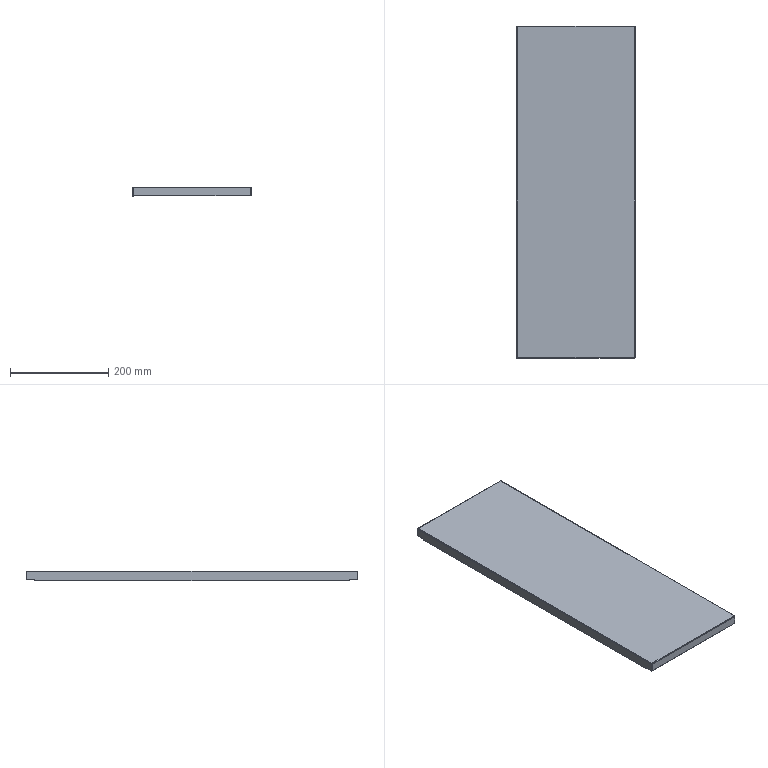Part | SolidWorks | features BaseBody 1 | 1 solid | 44 faces | box 239.8 x 674.5 x 20 mm | volume 231224 mm3 | plane 32 | cylinder 8 | spline 4 | commonest cylinder face diameters 1 x4 3.4 x4
STEP:
#1=CARTESIAN_POINT('',(-119.9,-337.25,-18.));
#2=VERTEX_POINT('',#1);
#3=CARTESIAN_POINT('',(-119.9,-319.25,-18.));
#4=VERTEX_POINT('',#3);
#5=CARTESIAN_POINT('',(-119.9,-337.25,-18.));
#6=DIRECTION('',(0.,1.,0.));
#7=VECTOR('',#6,1000.);
#8=LINE('',#5,#7);
#9=EDGE_CURVE('',#2,#4,#8,.T.);
#10=ORIENTED_EDGE('',*,*,#9,.T.);
#11=CARTESIAN_POINT('',(-118.7,-319.25,-18.));
#12=VERTEX_POINT('',#11);
#13=CARTESIAN_POINT('',(-118.7,-319.25,-18.));
#14=DIRECTION('',(-1.,0.,0.));
#15=VECTOR('',#14,1000.);
#16=LINE('',#13,#15);
#17=EDGE_CURVE('',#12,#4,#16,.T.);
#18=ORIENTED_EDGE('',*,*,#17,.F.);
#19=CARTESIAN_POINT('',(-118.7,-337.25,-18.));
#20=VERTEX_POINT('',#19);
#21=CARTESIAN_POINT('',(-118.7,-337.25,-18.));
#22=DIRECTION('',(0.,1.,0.));
#23=VECTOR('',#22,1000.);
#24=LINE('',#21,#23);
#25=EDGE_CURVE('',#20,#12,#24,.T.);
#26=ORIENTED_EDGE('',*,*,#25,.F.);
#27=CARTESIAN_POINT('',(-118.7,-337.25,-18.));
#28=DIRECTION('',(-1.,0.,0.));
#29=VECTOR('',#28,1000.);
#30=LINE('',#27,#29);
#31=EDGE_CURVE('',#20,#2,#30,.T.);
#32=ORIENTED_EDGE('',*,*,#31,.T.);
#33=EDGE_LOOP('',(#10,#18,#26,#32));
#34=FACE_OUTER_BOUND('',#33,.T.);
#35=CARTESIAN_POINT('',(-118.7,-337.25,-18.));
#36=DIRECTION('',(0.,0.,1.));
#37=DIRECTION('',(1.,0.,0.));
#38=AXIS2_PLACEMENT_3D('',#35,#36,#37);
#39=PLANE('',#38);
#40=ADVANCED_FACE('',(#34),#39,.F.);
#41=CARTESIAN_POINT('',(-119.9,-319.25,-20.));
#42=VERTEX_POINT('',#41);
#43=CARTESIAN_POINT('',(-119.9,-319.25,-20.));
#44=DIRECTION('',(0.,0.,-1.));
#45=VECTOR('',#44,1000.);
#46=LINE('',#43,#45);
#47=EDGE_CURVE('',#4,#42,#46,.T.);
#48=ORIENTED_EDGE('',*,*,#47,.T.);
#49=CARTESIAN_POINT('',(-118.7,-319.25,-20.));
#50=VERTEX_POINT('',#49);
#51=CARTESIAN_POINT('',(-118.7,-319.25,-20.));
#52=DIRECTION('',(-1.,0.,0.));
#53=VECTOR('',#52,1000.);
#54=LINE('',#51,#53);
#55=EDGE_CURVE('',#50,#42,#54,.T.);
#56=ORIENTED_EDGE('',*,*,#55,.F.);
#57=CARTESIAN_POINT('',(-118.7,-319.25,-20.));
#58=DIRECTION('',(0.,0.,-1.));
#59=VECTOR('',#58,1000.);
#60=LINE('',#57,#59);
#61=EDGE_CURVE('',#12,#50,#60,.T.);
#62=ORIENTED_EDGE('',*,*,#61,.F.);
#63=ORIENTED_EDGE('',*,*,#17,.T.);
#64=EDGE_LOOP('',(#48,#56,#62,#63));
#65=FACE_OUTER_BOUND('',#64,.T.);
#66=CARTESIAN_POINT('',(-118.7,-319.25,-20.));
#67=DIRECTION('',(0.,1.,0.));
#68=DIRECTION('',(1.,0.,0.));
#69=AXIS2_PLACEMENT_3D('',#66,#67,#68);
#70=PLANE('',#69);
#71=ADVANCED_FACE('',(#65),#70,.F.);
#72=CARTESIAN_POINT('',(-119.9,319.25,-20.));
#73=VERTEX_POINT('',#72);
#74=CARTESIAN_POINT('',(-119.9,319.25,-18.));
#75=VERTEX_POINT('',#74);
#76=CARTESIAN_POINT('',(-119.9,319.25,-20.));
#77=DIRECTION('',(0.,0.,1.));
#78=VECTOR('',#77,1000.);
#79=LINE('',#76,#78);
#80=EDGE_CURVE('',#73,#75,#79,.T.);
#81=ORIENTED_EDGE('',*,*,#80,.T.);
#82=CARTESIAN_POINT('',(-118.7,319.25,-18.));
#83=VERTEX_POINT('',#82);
#84=CARTESIAN_POINT('',(-118.7,319.25,-18.));
#85=DIRECTION('',(-1.,0.,0.));
#86=VECTOR('',#85,1000.);
#87=LINE('',#84,#86);
#88=EDGE_CURVE('',#83,#75,#87,.T.);
#89=ORIENTED_EDGE('',*,*,#88,.F.);
#90=CARTESIAN_POINT('',(-118.7,319.25,-20.));
#91=VERTEX_POINT('',#90);
#92=CARTESIAN_POINT('',(-118.7,319.25,-20.));
#93=DIRECTION('',(0.,0.,1.));
#94=VECTOR('',#93,1000.);
#95=LINE('',#92,#94);
#96=EDGE_CURVE('',#91,#83,#95,.T.);
#97=ORIENTED_EDGE('',*,*,#96,.F.);
#98=CARTESIAN_POINT('',(-118.7,319.25,-20.));
#99=DIRECTION('',(-1.,0.,0.));
#100=VECTOR('',#99,1000.);
#101=LINE('',#98,#100);
#102=EDGE_CURVE('',#91,#73,#101,.T.);
#103=ORIENTED_EDGE('',*,*,#102,.T.);
#104=EDGE_LOOP('',(#81,#89,#97,#103));
#105=FACE_OUTER_BOUND('',#104,.T.);
#106=CARTESIAN_POINT('',(-118.7,319.25,-20.));
#107=DIRECTION('',(0.,-1.,0.));
#108=DIRECTION('',(0.,0.,-1.));
#109=AXIS2_PLACEMENT_3D('',#106,#107,#108);
#110=PLANE('',#109);
#111=ADVANCED_FACE('',(#105),#110,.F.);
#112=CARTESIAN_POINT('',(-119.9,337.25,-18.));
#113=VERTEX_POINT('',#112);
#114=CARTESIAN_POINT('',(-119.9,337.25,-18.));
#115=DIRECTION('',(0.,1.,0.));
#116=VECTOR('',#115,1000.);
#117=LINE('',#114,#116);
#118=EDGE_CURVE('',#75,#113,#117,.T.);
#119=ORIENTED_EDGE('',*,*,#118,.T.);
#120=CARTESIAN_POINT('',(-118.7,337.25,-18.));
#121=VERTEX_POINT('',#120);
#122=CARTESIAN_POINT('',(-118.7,337.25,-18.));
#123=DIRECTION('',(-1.,0.,0.));
#124=VECTOR('',#123,1000.);
#125=LINE('',#122,#124);
#126=EDGE_CURVE('',#121,#113,#125,.T.);
#127=ORIENTED_EDGE('',*,*,#126,.F.);
#128=CARTESIAN_POINT('',(-118.7,337.25,-18.));
#129=DIRECTION('',(0.,1.,0.));
#130=VECTOR('',#129,1000.);
#131=LINE('',#128,#130);
#132=EDGE_CURVE('',#83,#121,#131,.T.);
#133=ORIENTED_EDGE('',*,*,#132,.F.);
#134=ORIENTED_EDGE('',*,*,#88,.T.);
#135=EDGE_LOOP('',(#119,#127,#133,#134));
#136=FACE_OUTER_BOUND('',#135,.T.);
#137=CARTESIAN_POINT('',(-118.7,337.25,-18.));
#138=DIRECTION('',(0.,0.,1.));
#139=DIRECTION('',(1.,0.,0.));
#140=AXIS2_PLACEMENT_3D('',#137,#138,#139);
#141=PLANE('',#140);
#142=ADVANCED_FACE('',(#136),#141,.F.);
#143=CARTESIAN_POINT('',(117.993,337.25,-18.));
#144=VERTEX_POINT('',#143);
#145=CARTESIAN_POINT('',(117.993,336.05,-18.));
#146=VERTEX_POINT('',#145);
#147=CARTESIAN_POINT('',(117.993,337.25,-18.));
#148=DIRECTION('',(0.,-1.,0.));
#149=VECTOR('',#148,1000.);
#150=LINE('',#147,#149);
#151=EDGE_CURVE('',#144,#146,#150,.T.);
#152=ORIENTED_EDGE('',*,*,#151,.F.);
#153=CARTESIAN_POINT('',(117.993,337.25,-1.7));
#154=VERTEX_POINT('',#153);
#155=CARTESIAN_POINT('',(117.993,337.25,0.));
#156=DIRECTION('',(0.,0.,-1.));
#157=VECTOR('',#156,1000.);
#158=LINE('',#155,#157);
#159=EDGE_CURVE('',#154,#144,#158,.T.);
#160=ORIENTED_EDGE('',*,*,#159,.F.);
#161=CARTESIAN_POINT('',(117.993,336.05,-1.7));
#162=VERTEX_POINT('',#161);
#163=CARTESIAN_POINT('',(117.993,336.05,-1.7));
#164=DIRECTION('',(0.,-1.,0.));
#165=VECTOR('',#164,1000.);
#166=LINE('',#163,#165);
#167=EDGE_CURVE('',#154,#162,#166,.T.);
#168=ORIENTED_EDGE('',*,*,#167,.T.);
#169=CARTESIAN_POINT('',(117.993,336.05,-1.2));
#170=DIRECTION('',(0.,0.,-1.));
#171=VECTOR('',#170,1000.);
#172=LINE('',#169,#171);
#173=EDGE_CURVE('',#162,#146,#172,.T.);
#174=ORIENTED_EDGE('',*,*,#173,.T.);
#175=EDGE_LOOP('',(#152,#160,#168,#174));
#176=FACE_OUTER_BOUND('',#175,.T.);
#177=CARTESIAN_POINT('',(117.993,336.05,-1.2));
#178=DIRECTION('',(-1.,0.,0.));
#179=DIRECTION('',(0.,0.,1.));
#180=AXIS2_PLACEMENT_3D('',#177,#178,#179);
#181=PLANE('',#180);
#182=ADVANCED_FACE('',(#176),#181,.F.);
#183=CARTESIAN_POINT('',(-118.2,337.25,-18.));
#184=VERTEX_POINT('',#183);
#185=CARTESIAN_POINT('',(0.,337.25,-18.));
#186=DIRECTION('',(-1.,0.,0.));
#187=VECTOR('',#186,1000.);
#188=LINE('',#185,#187);
#189=EDGE_CURVE('',#144,#184,#188,.T.);
#190=ORIENTED_EDGE('',*,*,#189,.F.);
#191=ORIENTED_EDGE('',*,*,#151,.T.);
#192=CARTESIAN_POINT('',(-118.2,336.05,-18.));
#193=VERTEX_POINT('',#192);
#194=CARTESIAN_POINT('',(-118.2,336.05,-18.));
#195=DIRECTION('',(-1.,0.,0.));
#196=VECTOR('',#195,1000.);
#197=LINE('',#194,#196);
#198=EDGE_CURVE('',#146,#193,#197,.T.);
#199=ORIENTED_EDGE('',*,*,#198,.T.);
#200=CARTESIAN_POINT('',(-118.2,337.25,-18.));
#201=DIRECTION('',(0.,-1.,0.));
#202=VECTOR('',#201,1000.);
#203=LINE('',#200,#202);
#204=EDGE_CURVE('',#184,#193,#203,.T.);
#205=ORIENTED_EDGE('',*,*,#204,.F.);
#206=EDGE_LOOP('',(#190,#191,#199,#205));
#207=FACE_OUTER_BOUND('',#206,.T.);
#208=CARTESIAN_POINT('',(-118.2,337.25,-18.));
#209=DIRECTION('',(0.,0.,1.));
#210=DIRECTION('',(0.,-1.,0.));
#211=AXIS2_PLACEMENT_3D('',#208,#209,#210);
#212=PLANE('',#211);
#213=ADVANCED_FACE('',(#207),#212,.F.);
#214=ORIENTED_EDGE('',*,*,#173,.F.);
#215=CARTESIAN_POINT('',(-118.2,336.05,-1.7));
#216=VERTEX_POINT('',#215);
#217=CARTESIAN_POINT('',(-118.2,336.05,-1.7));
#218=DIRECTION('',(1.,0.,0.));
#219=VECTOR('',#218,1000.);
#220=LINE('',#217,#219);
#221=EDGE_CURVE('',#216,#162,#220,.T.);
#222=ORIENTED_EDGE('',*,*,#221,.F.);
#223=CARTESIAN_POINT('',(-118.2,336.05,-1.2));
#224=DIRECTION('',(0.,0.,1.));
#225=VECTOR('',#224,1000.);
#226=LINE('',#223,#225);
#227=EDGE_CURVE('',#193,#216,#226,.T.);
#228=ORIENTED_EDGE('',*,*,#227,.F.);
#229=ORIENTED_EDGE('',*,*,#198,.F.);
#230=EDGE_LOOP('',(#214,#222,#228,#229));
#231=FACE_OUTER_BOUND('',#230,.T.);
#232=CARTESIAN_POINT('',(0.,336.05,0.));
#233=DIRECTION('',(0.,-1.,0.));
#234=DIRECTION('',(0.,0.,-1.));
#235=AXIS2_PLACEMENT_3D('',#232,#233,#234);
#236=PLANE('',#235);
#237=ADVANCED_FACE('',(#231),#236,.T.);
#238=CARTESIAN_POINT('',(-118.2,337.25,-1.7));
#239=VERTEX_POINT('',#238);
#240=CARTESIAN_POINT('',(-118.2,337.25,-1.7));
#241=DIRECTION('',(-1.,0.,0.));
#242=VECTOR('',#241,1000.);
#243=LINE('',#240,#242);
#244=EDGE_CURVE('',#154,#239,#243,.T.);
#245=ORIENTED_EDGE('',*,*,#244,.F.);
#246=ORIENTED_EDGE('',*,*,#159,.T.);
#247=ORIENTED_EDGE('',*,*,#189,.T.);
#248=CARTESIAN_POINT('',(-118.2,337.25,0.));
#249=DIRECTION('',(0.,0.,1.));
#250=VECTOR('',#249,1000.);
#251=LINE('',#248,#250);
#252=EDGE_CURVE('',#184,#239,#251,.T.);
#253=ORIENTED_EDGE('',*,*,#252,.T.);
#254=EDGE_LOOP('',(#245,#246,#247,#253));
#255=FACE_OUTER_BOUND('',#254,.T.);
#256=CARTESIAN_POINT('',(0.,337.25,0.));
#257=DIRECTION('',(0.,-1.,0.));
#258=DIRECTION('',(0.,0.,-1.));
#259=AXIS2_PLACEMENT_3D('',#256,#257,#258);
#260=PLANE('',#259);
#261=ADVANCED_FACE('',(#255),#260,.F.);
#262=CARTESIAN_POINT('',(-118.2,337.25,-1.7));
#263=DIRECTION('',(0.,1.,0.));
#264=VECTOR('',#263,1000.);
#265=LINE('',#262,#264);
#266=EDGE_CURVE('',#216,#239,#265,.T.);
#267=ORIENTED_EDGE('',*,*,#266,.T.);
#268=ORIENTED_EDGE('',*,*,#252,.F.);
#269=ORIENTED_EDGE('',*,*,#204,.T.);
#270=ORIENTED_EDGE('',*,*,#227,.T.);
#271=EDGE_LOOP('',(#267,#268,#269,#270));
#272=FACE_OUTER_BOUND('',#271,.T.);
#273=CARTESIAN_POINT('',(-118.2,337.25,-1.2));
#274=DIRECTION('',(1.,0.,0.));
#275=DIRECTION('',(0.,1.,0.));
#276=AXIS2_PLACEMENT_3D('',#273,#274,#275);
#277=PLANE('',#276);
#278=ADVANCED_FACE('',(#272),#277,.F.);
#279=CARTESIAN_POINT('',(118.2,335.55,-1.2));
#280=VERTEX_POINT('',#279);
#281=CARTESIAN_POINT('',(-118.2,335.55,-1.2));
#282=VERTEX_POINT('',#281);
#283=CARTESIAN_POINT('',(118.2,335.55,-1.2));
#284=DIRECTION('',(-1.,0.,0.));
#285=VECTOR('',#284,1000.);
#286=LINE('',#283,#285);
#287=EDGE_CURVE('',#280,#282,#286,.T.);
#288=ORIENTED_EDGE('',*,*,#287,.T.);
#289=CARTESIAN_POINT('',(-118.2,335.55,-1.7));
#290=DIRECTION('',(-1.,0.,0.));
#291=DIRECTION('',(0.,0.,-1.));
#292=AXIS2_PLACEMENT_3D('',#289,#290,#291);
#293=CIRCLE('',#292,0.5);
#294=EDGE_CURVE('',#282,#216,#293,.T.);
#295=ORIENTED_EDGE('',*,*,#294,.T.);
#296=ORIENTED_EDGE('',*,*,#221,.T.);
#297=CARTESIAN_POINT('',(117.993,336.05,-1.7));
#298=CARTESIAN_POINT('',(118.027,336.05,-1.569));
#299=CARTESIAN_POINT('',(118.062,335.996,-1.439));
#300=CARTESIAN_POINT('',(118.131,335.811,-1.254));
#301=CARTESIAN_POINT('',(118.165,335.681,-1.2));
#302=CARTESIAN_POINT('',(118.2,335.55,-1.2));
#303=B_SPLINE_CURVE_WITH_KNOTS('',3,(#297,#298,#299,#300,#301,#302),.UNSPECIFIED.,.F.,.F.,(4,2,4),(0.,0.5,1.),.UNSPECIFIED.);
#304=EDGE_CURVE('',#162,#280,#303,.T.);
#305=ORIENTED_EDGE('',*,*,#304,.T.);
#306=EDGE_LOOP('',(#288,#295,#296,#305));
#307=FACE_OUTER_BOUND('',#306,.T.);
#308=CARTESIAN_POINT('',(118.2,335.55,-1.7));
#309=DIRECTION('',(1.,0.,0.));
#310=DIRECTION('',(0.,1.,0.));
#311=AXIS2_PLACEMENT_3D('',#308,#309,#310);
#312=CYLINDRICAL_SURFACE('',#311,0.5);
#313=ADVANCED_FACE('',(#307),#312,.F.);
#314=CARTESIAN_POINT('',(118.2,335.55,0.));
#315=VERTEX_POINT('',#314);
#316=CARTESIAN_POINT('',(-118.2,335.55,0.));
#317=VERTEX_POINT('',#316);
#318=CARTESIAN_POINT('',(118.2,335.55,0.));
#319=DIRECTION('',(-1.,0.,0.));
#320=VECTOR('',#319,1000.);
#321=LINE('',#318,#320);
#322=EDGE_CURVE('',#315,#317,#321,.T.);
#323=ORIENTED_EDGE('',*,*,#322,.F.);
#324=CARTESIAN_POINT('',(117.993,337.25,-1.7));
#325=CARTESIAN_POINT('',(118.01,337.25,-1.477));
#326=CARTESIAN_POINT('',(118.027,337.206,-1.255));
#327=CARTESIAN_POINT('',(118.062,337.035,-0.8438));
#328=CARTESIAN_POINT('',(118.079,336.909,-0.6553));
#329=CARTESIAN_POINT('',(118.114,336.595,-0.3406));
#330=CARTESIAN_POINT('',(118.131,336.406,-0.2146));
#331=CARTESIAN_POINT('',(118.165,335.995,-0.04425));
#332=CARTESIAN_POINT('',(118.183,335.773,0.));
#333=CARTESIAN_POINT('',(118.2,335.55,0.));
#334=B_SPLINE_CURVE_WITH_KNOTS('',3,(#324,#325,#326,#327,#328,#329,#330,#331,#332,#333),.UNSPECIFIED.,.F.,.F.,(4,2,2,2,4),(0.,0.25,0.5,0.75,1.),.UNSPECIFIED.);
#335=EDGE_CURVE('',#154,#315,#334,.T.);
#336=ORIENTED_EDGE('',*,*,#335,.F.);
#337=ORIENTED_EDGE('',*,*,#244,.T.);
#338=CARTESIAN_POINT('',(-118.2,335.55,-1.7));
#339=DIRECTION('',(-1.,0.,0.));
#340=DIRECTION('',(0.,0.,-1.));
#341=AXIS2_PLACEMENT_3D('',#338,#339,#340);
#342=CIRCLE('',#341,1.7);
#343=EDGE_CURVE('',#317,#239,#342,.T.);
#344=ORIENTED_EDGE('',*,*,#343,.F.);
#345=EDGE_LOOP('',(#323,#336,#337,#344));
#346=FACE_OUTER_BOUND('',#345,.T.);
#347=CARTESIAN_POINT('',(118.2,335.55,-1.7));
#348=DIRECTION('',(1.,0.,0.));
#349=DIRECTION('',(0.,1.,0.));
#350=AXIS2_PLACEMENT_3D('',#347,#348,#349);
#351=CYLINDRICAL_SURFACE('',#350,1.7);
#352=ADVANCED_FACE('',(#346),#351,.T.);
#353=ORIENTED_EDGE('',*,*,#304,.F.);
#354=ORIENTED_EDGE('',*,*,#167,.F.);
#355=ORIENTED_EDGE('',*,*,#335,.T.);
#356=CARTESIAN_POINT('',(118.2,335.55,-1.2));
#357=DIRECTION('',(0.,0.,1.));
#358=VECTOR('',#357,1000.);
#359=LINE('',#356,#358);
#360=EDGE_CURVE('',#280,#315,#359,.T.);
#361=ORIENTED_EDGE('',*,*,#360,.F.);
#362=EDGE_LOOP('',(#353,#354,#355,#361));
#363=FACE_OUTER_BOUND('',#362,.T.);
#364=CARTESIAN_POINT('',(117.993,337.262,-1.7));
#365=CARTESIAN_POINT('',(118.01,337.262,-1.476));
#366=CARTESIAN_POINT('',(118.027,337.217,-1.252));
#367=CARTESIAN_POINT('',(118.062,337.046,-0.8378));
#368=CARTESIAN_POINT('',(118.079,336.919,-0.6479));
#369=CARTESIAN_POINT('',(118.114,336.602,-0.331));
#370=CARTESIAN_POINT('',(118.131,336.412,-0.2041));
#371=CARTESIAN_POINT('',(118.165,335.998,-0.03256));
#372=CARTESIAN_POINT('',(118.183,335.774,0.012));
#373=CARTESIAN_POINT('',(118.2,335.55,0.012));
#374=CARTESIAN_POINT('',(117.993,337.25,-1.7));
#375=CARTESIAN_POINT('',(118.01,337.25,-1.477));
#376=CARTESIAN_POINT('',(118.027,337.206,-1.255));
#377=CARTESIAN_POINT('',(118.062,337.035,-0.8438));
#378=CARTESIAN_POINT('',(118.079,336.909,-0.6553));
#379=CARTESIAN_POINT('',(118.114,336.595,-0.3406));
#380=CARTESIAN_POINT('',(118.131,336.406,-0.2146));
#381=CARTESIAN_POINT('',(118.165,335.995,-0.04425));
#382=CARTESIAN_POINT('',(118.183,335.773,0.));
#383=CARTESIAN_POINT('',(118.2,335.55,0.));
#384=CARTESIAN_POINT('',(117.993,336.05,-1.7));
#385=CARTESIAN_POINT('',(118.01,336.05,-1.635));
#386=CARTESIAN_POINT('',(118.027,336.037,-1.569));
#387=CARTESIAN_POINT('',(118.062,335.987,-1.448));
#388=CARTESIAN_POINT('',(118.079,335.95,-1.393));
#389=CARTESIAN_POINT('',(118.114,335.857,-1.3));
#390=CARTESIAN_POINT('',(118.131,335.802,-1.263));
#391=CARTESIAN_POINT('',(118.165,335.681,-1.213));
#392=CARTESIAN_POINT('',(118.183,335.615,-1.2));
#393=CARTESIAN_POINT('',(118.2,335.55,-1.2));
#394=CARTESIAN_POINT('',(117.993,336.038,-1.7));
#395=CARTESIAN_POINT('',(118.01,336.038,-1.636));
#396=CARTESIAN_POINT('',(118.027,336.025,-1.572));
#397=CARTESIAN_POINT('',(118.062,335.976,-1.454));
#398=CARTESIAN_POINT('',(118.079,335.94,-1.4));
#399=CARTESIAN_POINT('',(118.114,335.85,-1.31));
#400=CARTESIAN_POINT('',(118.131,335.796,-1.274));
#401=CARTESIAN_POINT('',(118.165,335.678,-1.225));
#402=CARTESIAN_POINT('',(118.183,335.614,-1.212));
#403=CARTESIAN_POINT('',(118.2,335.55,-1.212));
#404=B_SPLINE_SURFACE_WITH_KNOTS('',1,3,((#364,#365,#366,#367,#368,#369,#370,#371,#372,#373),(#374,#375,#376,#377,#378,#379,#380,#381,#382,#383),(#384,#385,#386,#387,#388,#389,#390,#391,#392,#393),(#394,#395,#396,#397,#398,#399,#400,#401,#402,#403)),.UNSPECIFIED.,.F.,.F.,.F.,(2,1,1,2),(4,2,2,2,4),(-0.01,0.,1.,1.01),(0.,0.25,0.5,0.75,1.),.UNSPECIFIED.);
#405=ADVANCED_FACE('',(#363),#404,.F.);
#406=ORIENTED_EDGE('',*,*,#266,.F.);
#407=ORIENTED_EDGE('',*,*,#294,.F.);
#408=CARTESIAN_POINT('',(-118.2,335.55,-1.2));
#409=DIRECTION('',(0.,0.,1.));
#410=VECTOR('',#409,1000.);
#411=LINE('',#408,#410);
#412=EDGE_CURVE('',#282,#317,#411,.T.);
#413=ORIENTED_EDGE('',*,*,#412,.T.);
#414=ORIENTED_EDGE('',*,*,#343,.T.);
#415=EDGE_LOOP('',(#406,#407,#413,#414));
#416=FACE_OUTER_BOUND('',#415,.T.);
#417=CARTESIAN_POINT('',(-118.2,335.55,-1.7));
#418=DIRECTION('',(-1.,0.,0.));
#419=DIRECTION('',(0.,0.,1.));
#420=AXIS2_PLACEMENT_3D('',#417,#418,#419);
#421=PLANE('',#420);
#422=ADVANCED_FACE('',(#416),#421,.T.);
#423=CARTESIAN_POINT('',(119.9,-335.343,-18.));
#424=VERTEX_POINT('',#423);
#425=CARTESIAN_POINT('',(118.7,-335.343,-18.));
#426=VERTEX_POINT('',#425);
#427=CARTESIAN_POINT('',(119.9,-335.343,-18.));
#428=DIRECTION('',(-1.,0.,0.));
#429=VECTOR('',#428,1000.);
#430=LINE('',#427,#429);
#431=EDGE_CURVE('',#424,#426,#430,.T.);
#432=ORIENTED_EDGE('',*,*,#431,.F.);
#433=CARTESIAN_POINT('',(119.9,-335.343,-1.7));
#434=VERTEX_POINT('',#433);
#435=CARTESIAN_POINT('',(119.9,-335.343,0.));
#436=DIRECTION('',(0.,0.,-1.));
#437=VECTOR('',#436,1000.);
#438=LINE('',#435,#437);
#439=EDGE_CURVE('',#434,#424,#438,.T.);
#440=ORIENTED_EDGE('',*,*,#439,.F.);
#441=CARTESIAN_POINT('',(118.7,-335.343,-1.7));
#442=VERTEX_POINT('',#441);
#443=CARTESIAN_POINT('',(118.7,-335.343,-1.7));
#444=DIRECTION('',(-1.,0.,0.));
#445=VECTOR('',#444,1000.);
#446=LINE('',#443,#445);
#447=EDGE_CURVE('',#434,#442,#446,.T.);
#448=ORIENTED_EDGE('',*,*,#447,.T.);
#449=CARTESIAN_POINT('',(118.7,-335.343,-1.2));
#450=DIRECTION('',(0.,0.,-1.));
#451=VECTOR('',#450,1000.);
#452=LINE('',#449,#451);
#453=EDGE_CURVE('',#442,#426,#452,.T.);
#454=ORIENTED_EDGE('',*,*,#453,.T.);
#455=EDGE_LOOP('',(#432,#440,#448,#454));
#456=FACE_OUTER_BOUND('',#455,.T.);
#457=CARTESIAN_POINT('',(118.7,-335.343,-1.2));
#458=DIRECTION('',(0.,1.,0.));
#459=DIRECTION('',(0.,0.,-1.));
#460=AXIS2_PLACEMENT_3D('',#457,#458,#459);
#461=PLANE('',#460);
#462=ADVANCED_FACE('',(#456),#461,.F.);
#463=CARTESIAN_POINT('',(119.9,335.343,-18.));
#464=VERTEX_POINT('',#463);
#465=CARTESIAN_POINT('',(118.7,335.343,-18.));
#466=VERTEX_POINT('',#465);
#467=CARTESIAN_POINT('',(118.7,335.343,-18.));
#468=DIRECTION('',(-1.,0.,0.));
#469=VECTOR('',#468,1000.);
#470=LINE('',#467,#469);
#471=EDGE_CURVE('',#464,#466,#470,.T.);
#472=ORIENTED_EDGE('',*,*,#471,.F.);
#473=CARTESIAN_POINT('',(119.9,0.,-18.));
#474=DIRECTION('',(0.,1.,0.));
#475=VECTOR('',#474,1000.);
#476=LINE('',#473,#475);
#477=EDGE_CURVE('',#424,#464,#476,.T.);
#478=ORIENTED_EDGE('',*,*,#477,.F.);
#479=ORIENTED_EDGE('',*,*,#431,.T.);
#480=CARTESIAN_POINT('',(118.7,337.25,-18.));
#481=DIRECTION('',(0.,1.,0.));
#482=VECTOR('',#481,1000.);
#483=LINE('',#480,#482);
#484=EDGE_CURVE('',#426,#466,#483,.T.);
#485=ORIENTED_EDGE('',*,*,#484,.T.);
#486=EDGE_LOOP('',(#472,#478,#479,#485));
#487=FACE_OUTER_BOUND('',#486,.T.);
#488=CARTESIAN_POINT('',(119.9,337.25,-18.));
#489=DIRECTION('',(0.,0.,1.));
#490=DIRECTION('',(1.,0.,0.));
#491=AXIS2_PLACEMENT_3D('',#488,#489,#490);
#492=PLANE('',#491);
#493=ADVANCED_FACE('',(#487),#492,.F.);
#494=CARTESIAN_POINT('',(118.7,335.343,-1.7));
#495=VERTEX_POINT('',#494);
#496=CARTESIAN_POINT('',(118.7,337.25,-1.7));
#497=DIRECTION('',(0.,-1.,0.));
#498=VECTOR('',#497,1000.);
#499=LINE('',#496,#498);
#500=EDGE_CURVE('',#495,#442,#499,.T.);
#501=ORIENTED_EDGE('',*,*,#500,.F.);
#502=CARTESIAN_POINT('',(118.7,335.343,0.));
#503=DIRECTION('',(0.,0.,-1.));
#504=VECTOR('',#503,1000.);
#505=LINE('',#502,#504);
#506=EDGE_CURVE('',#495,#466,#505,.T.);
#507=ORIENTED_EDGE('',*,*,#506,.T.);
#508=ORIENTED_EDGE('',*,*,#484,.F.);
#509=ORIENTED_EDGE('',*,*,#453,.F.);
#510=EDGE_LOOP('',(#501,#507,#508,#509));
#511=FACE_OUTER_BOUND('',#510,.T.);
#512=CARTESIAN_POINT('',(118.7,0.,0.));
#513=DIRECTION('',(-1.,0.,0.));
#514=DIRECTION('',(0.,0.,1.));
#515=AXIS2_PLACEMENT_3D('',#512,#513,#514);
#516=PLANE('',#515);
#517=ADVANCED_FACE('',(#511),#516,.T.);
#518=CARTESIAN_POINT('',(119.9,335.343,-1.7));
#519=VERTEX_POINT('',#518);
#520=CARTESIAN_POINT('',(119.9,335.343,-1.2));
#521=DIRECTION('',(0.,0.,-1.));
#522=VECTOR('',#521,1000.);
#523=LINE('',#520,#522);
#524=EDGE_CURVE('',#519,#464,#523,.T.);
#525=ORIENTED_EDGE('',*,*,#524,.F.);
#526=CARTESIAN_POINT('',(119.9,337.25,-1.7));
#527=DIRECTION('',(0.,1.,0.));
#528=VECTOR('',#527,1000.);
#529=LINE('',#526,#528);
#530=EDGE_CURVE('',#434,#519,#529,.T.);
#531=ORIENTED_EDGE('',*,*,#530,.F.);
#532=ORIENTED_EDGE('',*,*,#439,.T.);
#533=ORIENTED_EDGE('',*,*,#477,.T.);
#534=EDGE_LOOP('',(#525,#531,#532,#533));
#535=FACE_OUTER_BOUND('',#534,.T.);
#536=CARTESIAN_POINT('',(119.9,0.,0.));
#537=DIRECTION('',(-1.,0.,0.));
#538=DIRECTION('',(0.,0.,1.));
#539=AXIS2_PLACEMENT_3D('',#536,#537,#538);
#540=PLANE('',#539);
#541=ADVANCED_FACE('',(#535),#540,.F.);
#542=ORIENTED_EDGE('',*,*,#524,.T.);
#543=ORIENTED_EDGE('',*,*,#471,.T.);
#544=ORIENTED_EDGE('',*,*,#506,.F.);
#545=CARTESIAN_POINT('',(118.7,335.343,-1.7));
#546=DIRECTION('',(-1.,0.,0.));
#547=VECTOR('',#546,1000.);
#548=LINE('',#545,#547);
#549=EDGE_CURVE('',#519,#495,#548,.T.);
#550=ORIENTED_EDGE('',*,*,#549,.F.);
#551=EDGE_LOOP('',(#542,#543,#544,#550));
#552=FACE_OUTER_BOUND('',#551,.T.);
#553=CARTESIAN_POINT('',(118.7,335.343,-1.2));
#554=DIRECTION('',(0.,1.,0.));
#555=DIRECTION('',(0.,0.,-1.));
#556=AXIS2_PLACEMENT_3D('',#553,#554,#555);
#557=PLANE('',#556);
#558=ADVANCED_FACE('',(#552),#557,.T.);
#559=CARTESIAN_POINT('',(118.2,-335.55,-1.2));
#560=VERTEX_POINT('',#559);
#561=CARTESIAN_POINT('',(118.2,-335.55,-1.2));
#562=DIRECTION('',(0.,1.,0.));
#563=VECTOR('',#562,1000.);
#564=LINE('',#561,#563);
#565=EDGE_CURVE('',#560,#280,#564,.T.);
#566=ORIENTED_EDGE('',*,*,#565,.T.);
#567=CARTESIAN_POINT('',(118.2,335.55,-1.2));
#568=CARTESIAN_POINT('',(118.331,335.515,-1.2));
#569=CARTESIAN_POINT('',(118.461,335.481,-1.254));
#570=CARTESIAN_POINT('',(118.646,335.412,-1.439));
#571=CARTESIAN_POINT('',(118.7,335.377,-1.569));
#572=CARTESIAN_POINT('',(118.7,335.343,-1.7));
#573=B_SPLINE_CURVE_WITH_KNOTS('',3,(#567,#568,#569,#570,#571,#572),.UNSPECIFIED.,.F.,.F.,(4,2,4),(0.,0.5,1.),.UNSPECIFIED.);
#574=EDGE_CURVE('',#280,#495,#573,.T.);
#575=ORIENTED_EDGE('',*,*,#574,.T.);
#576=ORIENTED_EDGE('',*,*,#500,.T.);
#577=CARTESIAN_POINT('',(118.7,-335.343,-1.7));
#578=CARTESIAN_POINT('',(118.7,-335.377,-1.569));
#579=CARTESIAN_POINT('',(118.646,-335.412,-1.439));
#580=CARTESIAN_POINT('',(118.461,-335.481,-1.254));
#581=CARTESIAN_POINT('',(118.331,-335.515,-1.2));
#582=CARTESIAN_POINT('',(118.2,-335.55,-1.2));
#583=B_SPLINE_CURVE_WITH_KNOTS('',3,(#577,#578,#579,#580,#581,#582),.UNSPECIFIED.,.F.,.F.,(4,2,4),(0.,0.5,1.),.UNSPECIFIED.);
#584=EDGE_CURVE('',#442,#560,#583,.T.);
#585=ORIENTED_EDGE('',*,*,#584,.T.);
#586=EDGE_LOOP('',(#566,#575,#576,#585));
#587=FACE_OUTER_BOUND('',#586,.T.);
#588=CARTESIAN_POINT('',(118.2,-335.55,-1.7));
#589=DIRECTION('',(0.,-1.,0.));
#590=DIRECTION('',(1.,0.,0.));
#591=AXIS2_PLACEMENT_3D('',#588,#589,#590);
#592=CYLINDRICAL_SURFACE('',#591,0.5);
#593=ADVANCED_FACE('',(#587),#592,.F.);
#594=CARTESIAN_POINT('',(118.2,-335.55,0.));
#595=VERTEX_POINT('',#594);
#596=CARTESIAN_POINT('',(118.2,-335.55,0.));
#597=DIRECTION('',(0.,1.,0.));
#598=VECTOR('',#597,1000.);
#599=LINE('',#596,#598);
#600=EDGE_CURVE('',#595,#315,#599,.T.);
#601=ORIENTED_EDGE('',*,*,#600,.F.);
#602=CARTESIAN_POINT('',(119.9,-335.343,-1.7));
#603=CARTESIAN_POINT('',(119.9,-335.36,-1.477));
#604=CARTESIAN_POINT('',(119.856,-335.377,-1.255));
#605=CARTESIAN_POINT('',(119.685,-335.412,-0.8438));
#606=CARTESIAN_POINT('',(119.559,-335.429,-0.6553));
#607=CARTESIAN_POINT('',(119.245,-335.464,-0.3406));
#608=CARTESIAN_POINT('',(119.056,-335.481,-0.2146));
#609=CARTESIAN_POINT('',(118.645,-335.515,-0.04425));
#610=CARTESIAN_POINT('',(118.423,-335.533,0.));
#611=CARTESIAN_POINT('',(118.2,-335.55,0.));
#612=B_SPLINE_CURVE_WITH_KNOTS('',3,(#602,#603,#604,#605,#606,#607,#608,#609,#610,#611),.UNSPECIFIED.,.F.,.F.,(4,2,2,2,4),(0.,0.25,0.5,0.75,1.),.UNSPECIFIED.);
#613=EDGE_CURVE('',#434,#595,#612,.T.);
#614=ORIENTED_EDGE('',*,*,#613,.F.);
#615=ORIENTED_EDGE('',*,*,#530,.T.);
#616=CARTESIAN_POINT('',(118.2,335.55,0.));
#617=CARTESIAN_POINT('',(118.423,335.533,0.));
#618=CARTESIAN_POINT('',(118.645,335.515,-0.04425));
#619=CARTESIAN_POINT('',(119.056,335.481,-0.2146));
#620=CARTESIAN_POINT('',(119.245,335.464,-0.3406));
#621=CARTESIAN_POINT('',(119.559,335.429,-0.6553));
#622=CARTESIAN_POINT('',(119.685,335.412,-0.8438));
#623=CARTESIAN_POINT('',(119.856,335.377,-1.255));
#624=CARTESIAN_POINT('',(119.9,335.36,-1.477));
#625=CARTESIAN_POINT('',(119.9,335.343,-1.7));
#626=B_SPLINE_CURVE_WITH_KNOTS('',3,(#616,#617,#618,#619,#620,#621,#622,#623,#624,#625),.UNSPECIFIED.,.F.,.F.,(4,2,2,2,4),(0.,0.25,0.5,0.75,1.),.UNSPECIFIED.);
#627=EDGE_CURVE('',#315,#519,#626,.T.);
#628=ORIENTED_EDGE('',*,*,#627,.F.);
#629=EDGE_LOOP('',(#601,#614,#615,#628));
#630=FACE_OUTER_BOUND('',#629,.T.);
#631=CARTESIAN_POINT('',(118.2,-335.55,-1.7));
#632=DIRECTION('',(0.,-1.,0.));
#633=DIRECTION('',(1.,0.,0.));
#634=AXIS2_PLACEMENT_3D('',#631,#632,#633);
#635=CYLINDRICAL_SURFACE('',#634,1.7);
#636=ADVANCED_FACE('',(#630),#635,.T.);
#637=ORIENTED_EDGE('',*,*,#584,.F.);
#638=ORIENTED_EDGE('',*,*,#447,.F.);
#639=ORIENTED_EDGE('',*,*,#613,.T.);
#640=CARTESIAN_POINT('',(118.2,-335.55,-1.2));
#641=DIRECTION('',(0.,0.,1.));
#642=VECTOR('',#641,1000.);
#643=LINE('',#640,#642);
#644=EDGE_CURVE('',#560,#595,#643,.T.);
#645=ORIENTED_EDGE('',*,*,#644,.F.);
#646=EDGE_LOOP('',(#637,#638,#639,#645));
#647=FACE_OUTER_BOUND('',#646,.T.);
#648=CARTESIAN_POINT('',(119.912,-335.343,-1.7));
#649=CARTESIAN_POINT('',(119.912,-335.36,-1.476));
#650=CARTESIAN_POINT('',(119.867,-335.377,-1.252));
#651=CARTESIAN_POINT('',(119.696,-335.412,-0.8378));
#652=CARTESIAN_POINT('',(119.569,-335.429,-0.6479));
#653=CARTESIAN_POINT('',(119.252,-335.464,-0.331));
#654=CARTESIAN_POINT('',(119.062,-335.481,-0.2041));
#655=CARTESIAN_POINT('',(118.648,-335.515,-0.03256));
#656=CARTESIAN_POINT('',(118.424,-335.533,0.012));
#657=CARTESIAN_POINT('',(118.2,-335.55,0.012));
#658=CARTESIAN_POINT('',(119.9,-335.343,-1.7));
#659=CARTESIAN_POINT('',(119.9,-335.36,-1.477));
#660=CARTESIAN_POINT('',(119.856,-335.377,-1.255));
#661=CARTESIAN_POINT('',(119.685,-335.412,-0.8438));
#662=CARTESIAN_POINT('',(119.559,-335.429,-0.6553));
#663=CARTESIAN_POINT('',(119.245,-335.464,-0.3406));
#664=CARTESIAN_POINT('',(119.056,-335.481,-0.2146));
#665=CARTESIAN_POINT('',(118.645,-335.515,-0.04425));
#666=CARTESIAN_POINT('',(118.423,-335.533,0.));
#667=CARTESIAN_POINT('',(118.2,-335.55,0.));
#668=CARTESIAN_POINT('',(118.7,-335.343,-1.7));
#669=CARTESIAN_POINT('',(118.7,-335.36,-1.635));
#670=CARTESIAN_POINT('',(118.687,-335.377,-1.569));
#671=CARTESIAN_POINT('',(118.637,-335.412,-1.448));
#672=CARTESIAN_POINT('',(118.6,-335.429,-1.393));
#673=CARTESIAN_POINT('',(118.507,-335.464,-1.3));
#674=CARTESIAN_POINT('',(118.452,-335.481,-1.263));
#675=CARTESIAN_POINT('',(118.331,-335.515,-1.213));
#676=CARTESIAN_POINT('',(118.265,-335.533,-1.2));
#677=CARTESIAN_POINT('',(118.2,-335.55,-1.2));
#678=CARTESIAN_POINT('',(118.688,-335.343,-1.7));
#679=CARTESIAN_POINT('',(118.688,-335.36,-1.636));
#680=CARTESIAN_POINT('',(118.675,-335.377,-1.572));
#681=CARTESIAN_POINT('',(118.626,-335.412,-1.454));
#682=CARTESIAN_POINT('',(118.59,-335.429,-1.4));
#683=CARTESIAN_POINT('',(118.5,-335.464,-1.31));
#684=CARTESIAN_POINT('',(118.446,-335.481,-1.274));
#685=CARTESIAN_POINT('',(118.328,-335.515,-1.225));
#686=CARTESIAN_POINT('',(118.264,-335.533,-1.212));
#687=CARTESIAN_POINT('',(118.2,-335.55,-1.212));
#688=B_SPLINE_SURFACE_WITH_KNOTS('',1,3,((#648,#649,#650,#651,#652,#653,#654,#655,#656,#657),(#658,#659,#660,#661,#662,#663,#664,#665,#666,#667),(#668,#669,#670,#671,#672,#673,#674,#675,#676,#677),(#678,#679,#680,#681,#682,#683,#684,#685,#686,#687)),.UNSPECIFIED.,.F.,.F.,.F.,(2,1,1,2),(4,2,2,2,4),(-0.01,0.,1.,1.01),(0.,0.25,0.5,0.75,1.),.UNSPECIFIED.);
#689=ADVANCED_FACE('',(#647),#688,.F.);
#690=ORIENTED_EDGE('',*,*,#549,.T.);
#691=ORIENTED_EDGE('',*,*,#574,.F.);
#692=ORIENTED_EDGE('',*,*,#360,.T.);
#693=ORIENTED_EDGE('',*,*,#627,.T.);
#694=EDGE_LOOP('',(#690,#691,#692,#693));
#695=FACE_OUTER_BOUND('',#694,.T.);
#696=CARTESIAN_POINT('',(118.2,335.55,0.012));
#697=CARTESIAN_POINT('',(118.424,335.533,0.012));
#698=CARTESIAN_POINT('',(118.648,335.515,-0.03256));
#699=CARTESIAN_POINT('',(119.062,335.481,-0.2041));
#700=CARTESIAN_POINT('',(119.252,335.464,-0.331));
#701=CARTESIAN_POINT('',(119.569,335.429,-0.6479));
#702=CARTESIAN_POINT('',(119.696,335.412,-0.8378));
#703=CARTESIAN_POINT('',(119.867,335.377,-1.252));
#704=CARTESIAN_POINT('',(119.912,335.36,-1.476));
#705=CARTESIAN_POINT('',(119.912,335.343,-1.7));
#706=CARTESIAN_POINT('',(118.2,335.55,0.));
#707=CARTESIAN_POINT('',(118.423,335.533,0.));
#708=CARTESIAN_POINT('',(118.645,335.515,-0.04425));
#709=CARTESIAN_POINT('',(119.056,335.481,-0.2146));
#710=CARTESIAN_POINT('',(119.245,335.464,-0.3406));
#711=CARTESIAN_POINT('',(119.559,335.429,-0.6553));
#712=CARTESIAN_POINT('',(119.685,335.412,-0.8438));
#713=CARTESIAN_POINT('',(119.856,335.377,-1.255));
#714=CARTESIAN_POINT('',(119.9,335.36,-1.477));
#715=CARTESIAN_POINT('',(119.9,335.343,-1.7));
#716=CARTESIAN_POINT('',(118.2,335.55,-1.2));
#717=CARTESIAN_POINT('',(118.265,335.533,-1.2));
#718=CARTESIAN_POINT('',(118.331,335.515,-1.213));
#719=CARTESIAN_POINT('',(118.452,335.481,-1.263));
#720=CARTESIAN_POINT('',(118.507,335.464,-1.3));
#721=CARTESIAN_POINT('',(118.6,335.429,-1.393));
#722=CARTESIAN_POINT('',(118.637,335.412,-1.448));
#723=CARTESIAN_POINT('',(118.687,335.377,-1.569));
#724=CARTESIAN_POINT('',(118.7,335.36,-1.635));
#725=CARTESIAN_POINT('',(118.7,335.343,-1.7));
#726=CARTESIAN_POINT('',(118.2,335.55,-1.212));
#727=CARTESIAN_POINT('',(118.264,335.533,-1.212));
#728=CARTESIAN_POINT('',(118.328,335.515,-1.225));
#729=CARTESIAN_POINT('',(118.446,335.481,-1.274));
#730=CARTESIAN_POINT('',(118.5,335.464,-1.31));
#731=CARTESIAN_POINT('',(118.59,335.429,-1.4));
#732=CARTESIAN_POINT('',(118.626,335.412,-1.454));
#733=CARTESIAN_POINT('',(118.675,335.377,-1.572));
#734=CARTESIAN_POINT('',(118.688,335.36,-1.636));
#735=CARTESIAN_POINT('',(118.688,335.343,-1.7));
#736=B_SPLINE_SURFACE_WITH_KNOTS('',1,3,((#696,#697,#698,#699,#700,#701,#702,#703,#704,#705),(#706,#707,#708,#709,#710,#711,#712,#713,#714,#715),(#716,#717,#718,#719,#720,#721,#722,#723,#724,#725),(#726,#727,#728,#729,#730,#731,#732,#733,#734,#735)),.UNSPECIFIED.,.F.,.F.,.F.,(2,1,1,2),(4,2,2,2,4),(-0.01,0.,1.,1.01),(0.,0.25,0.5,0.75,1.),.UNSPECIFIED.);
#737=ADVANCED_FACE('',(#695),#736,.F.);
#738=CARTESIAN_POINT('',(-118.2,-336.05,-1.7));
#739=VERTEX_POINT('',#738);
#740=CARTESIAN_POINT('',(-118.2,-337.25,-1.7));
#741=VERTEX_POINT('',#740);
#742=CARTESIAN_POINT('',(-118.2,-336.05,-1.7));
#743=DIRECTION('',(0.,-1.,0.));
#744=VECTOR('',#743,1000.);
#745=LINE('',#742,#744);
#746=EDGE_CURVE('',#739,#741,#745,.T.);
#747=ORIENTED_EDGE('',*,*,#746,.F.);
#748=CARTESIAN_POINT('',(-118.2,-336.05,-18.));
#749=VERTEX_POINT('',#748);
#750=CARTESIAN_POINT('',(-118.2,-336.05,-18.));
#751=DIRECTION('',(0.,0.,-1.));
#752=VECTOR('',#751,1000.);
#753=LINE('',#750,#752);
#754=EDGE_CURVE('',#739,#749,#753,.T.);
#755=ORIENTED_EDGE('',*,*,#754,.T.);
#756=CARTESIAN_POINT('',(-118.2,-337.25,-18.));
#757=VERTEX_POINT('',#756);
#758=CARTESIAN_POINT('',(-118.2,-337.25,-18.));
#759=DIRECTION('',(0.,1.,0.));
#760=VECTOR('',#759,1000.);
#761=LINE('',#758,#760);
#762=EDGE_CURVE('',#757,#749,#761,.T.);
#763=ORIENTED_EDGE('',*,*,#762,.F.);
#764=CARTESIAN_POINT('',(-118.2,-337.25,0.));
#765=DIRECTION('',(0.,0.,-1.));
#766=VECTOR('',#765,1000.);
#767=LINE('',#764,#766);
#768=EDGE_CURVE('',#741,#757,#767,.T.);
#769=ORIENTED_EDGE('',*,*,#768,.F.);
#770=EDGE_LOOP('',(#747,#755,#763,#769));
#771=FACE_OUTER_BOUND('',#770,.T.);
#772=CARTESIAN_POINT('',(-118.2,-337.25,-18.));
#773=DIRECTION('',(1.,0.,0.));
#774=DIRECTION('',(0.,0.,1.));
#775=AXIS2_PLACEMENT_3D('',#772,#773,#774);
#776=PLANE('',#775);
#777=ADVANCED_FACE('',(#771),#776,.F.);
#778=CARTESIAN_POINT('',(117.993,-337.25,-18.));
#779=VERTEX_POINT('',#778);
#780=CARTESIAN_POINT('',(117.993,-336.05,-18.));
#781=VERTEX_POINT('',#780);
#782=CARTESIAN_POINT('',(117.993,-336.05,-18.));
#783=DIRECTION('',(0.,1.,0.));
#784=VECTOR('',#783,1000.);
#785=LINE('',#782,#784);
#786=EDGE_CURVE('',#779,#781,#785,.T.);
#787=ORIENTED_EDGE('',*,*,#786,.F.);
#788=CARTESIAN_POINT('',(0.,-337.25,-18.));
#789=DIRECTION('',(1.,0.,0.));
#790=VECTOR('',#789,1000.);
#791=LINE('',#788,#790);
#792=EDGE_CURVE('',#757,#779,#791,.T.);
#793=ORIENTED_EDGE('',*,*,#792,.F.);
#794=ORIENTED_EDGE('',*,*,#762,.T.);
#795=CARTESIAN_POINT('',(119.9,-336.05,-18.));
#796=DIRECTION('',(1.,0.,0.));
#797=VECTOR('',#796,1000.);
#798=LINE('',#795,#797);
#799=EDGE_CURVE('',#749,#781,#798,.T.);
#800=ORIENTED_EDGE('',*,*,#799,.T.);
#801=EDGE_LOOP('',(#787,#793,#794,#800));
#802=FACE_OUTER_BOUND('',#801,.T.);
#803=CARTESIAN_POINT('',(119.9,-337.25,-18.));
#804=DIRECTION('',(0.,0.,1.));
#805=DIRECTION('',(0.,-1.,0.));
#806=AXIS2_PLACEMENT_3D('',#803,#804,#805);
#807=PLANE('',#806);
#808=ADVANCED_FACE('',(#802),#807,.F.);
#809=CARTESIAN_POINT('',(117.993,-336.05,-1.7));
#810=VERTEX_POINT('',#809);
#811=CARTESIAN_POINT('',(119.9,-336.05,-1.7));
#812=DIRECTION('',(-1.,0.,0.));
#813=VECTOR('',#812,1000.);
#814=LINE('',#811,#813);
#815=EDGE_CURVE('',#810,#739,#814,.T.);
#816=ORIENTED_EDGE('',*,*,#815,.F.);
#817=CARTESIAN_POINT('',(117.993,-336.05,0.));
#818=DIRECTION('',(0.,0.,-1.));
#819=VECTOR('',#818,1000.);
#820=LINE('',#817,#819);
#821=EDGE_CURVE('',#810,#781,#820,.T.);
#822=ORIENTED_EDGE('',*,*,#821,.T.);
#823=ORIENTED_EDGE('',*,*,#799,.F.);
#824=ORIENTED_EDGE('',*,*,#754,.F.);
#825=EDGE_LOOP('',(#816,#822,#823,#824));
#826=FACE_OUTER_BOUND('',#825,.T.);
#827=CARTESIAN_POINT('',(0.,-336.05,0.));
#828=DIRECTION('',(0.,1.,0.));
#829=DIRECTION('',(0.,0.,-1.));
#830=AXIS2_PLACEMENT_3D('',#827,#828,#829);
#831=PLANE('',#830);
#832=ADVANCED_FACE('',(#826),#831,.T.);
#833=CARTESIAN_POINT('',(117.993,-337.25,-1.7));
#834=VERTEX_POINT('',#833);
#835=CARTESIAN_POINT('',(117.993,-337.25,-1.2));
#836=DIRECTION('',(0.,0.,-1.));
#837=VECTOR('',#836,1000.);
#838=LINE('',#835,#837);
#839=EDGE_CURVE('',#834,#779,#838,.T.);
#840=ORIENTED_EDGE('',*,*,#839,.F.);
#841=CARTESIAN_POINT('',(119.9,-337.25,-1.7));
#842=DIRECTION('',(1.,0.,0.));
#843=VECTOR('',#842,1000.);
#844=LINE('',#841,#843);
#845=EDGE_CURVE('',#741,#834,#844,.T.);
#846=ORIENTED_EDGE('',*,*,#845,.F.);
#847=ORIENTED_EDGE('',*,*,#768,.T.);
#848=ORIENTED_EDGE('',*,*,#792,.T.);
#849=EDGE_LOOP('',(#840,#846,#847,#848));
#850=FACE_OUTER_BOUND('',#849,.T.);
#851=CARTESIAN_POINT('',(0.,-337.25,0.));
#852=DIRECTION('',(0.,1.,0.));
#853=DIRECTION('',(0.,0.,-1.));
#854=AXIS2_PLACEMENT_3D('',#851,#852,#853);
#855=PLANE('',#854);
#856=ADVANCED_FACE('',(#850),#855,.F.);
#857=ORIENTED_EDGE('',*,*,#839,.T.);
#858=ORIENTED_EDGE('',*,*,#786,.T.);
#859=ORIENTED_EDGE('',*,*,#821,.F.);
#860=CARTESIAN_POINT('',(117.993,-336.05,-1.7));
#861=DIRECTION('',(0.,1.,0.));
#862=VECTOR('',#861,1000.);
#863=LINE('',#860,#862);
#864=EDGE_CURVE('',#834,#810,#863,.T.);
#865=ORIENTED_EDGE('',*,*,#864,.F.);
#866=EDGE_LOOP('',(#857,#858,#859,#865));
#867=FACE_OUTER_BOUND('',#866,.T.);
#868=CARTESIAN_POINT('',(117.993,-336.05,-1.2));
#869=DIRECTION('',(1.,0.,0.));
#870=DIRECTION('',(0.,1.,0.));
#871=AXIS2_PLACEMENT_3D('',#868,#869,#870);
#872=PLANE('',#871);
#873=ADVANCED_FACE('',(#867),#872,.T.);
#874=CARTESIAN_POINT('',(-118.2,-335.55,-1.2));
#875=VERTEX_POINT('',#874);
#876=CARTESIAN_POINT('',(-118.2,-335.55,-1.2));
#877=DIRECTION('',(1.,0.,0.));
#878=VECTOR('',#877,1000.);
#879=LINE('',#876,#878);
#880=EDGE_CURVE('',#875,#560,#879,.T.);
#881=ORIENTED_EDGE('',*,*,#880,.T.);
#882=CARTESIAN_POINT('',(118.2,-335.55,-1.2));
#883=CARTESIAN_POINT('',(118.165,-335.681,-1.2));
#884=CARTESIAN_POINT('',(118.131,-335.811,-1.254));
#885=CARTESIAN_POINT('',(118.062,-335.996,-1.439));
#886=CARTESIAN_POINT('',(118.027,-336.05,-1.569));
#887=CARTESIAN_POINT('',(117.993,-336.05,-1.7));
#888=B_SPLINE_CURVE_WITH_KNOTS('',3,(#882,#883,#884,#885,#886,#887),.UNSPECIFIED.,.F.,.F.,(4,2,4),(0.,0.5,1.),.UNSPECIFIED.);
#889=EDGE_CURVE('',#560,#810,#888,.T.);
#890=ORIENTED_EDGE('',*,*,#889,.T.);
#891=ORIENTED_EDGE('',*,*,#815,.T.);
#892=CARTESIAN_POINT('',(-118.2,-335.55,-1.7));
#893=DIRECTION('',(-1.,0.,0.));
#894=DIRECTION('',(0.,0.,1.));
#895=AXIS2_PLACEMENT_3D('',#892,#893,#894);
#896=CIRCLE('',#895,0.5);
#897=EDGE_CURVE('',#739,#875,#896,.T.);
#898=ORIENTED_EDGE('',*,*,#897,.T.);
#899=EDGE_LOOP('',(#881,#890,#891,#898));
#900=FACE_OUTER_BOUND('',#899,.T.);
#901=CARTESIAN_POINT('',(-118.2,-335.55,-1.7));
#902=DIRECTION('',(-1.,0.,0.));
#903=DIRECTION('',(0.,-1.,0.));
#904=AXIS2_PLACEMENT_3D('',#901,#902,#903);
#905=CYLINDRICAL_SURFACE('',#904,0.5);
#906=ADVANCED_FACE('',(#900),#905,.F.);
#907=CARTESIAN_POINT('',(-118.2,-335.55,0.));
#908=VERTEX_POINT('',#907);
#909=CARTESIAN_POINT('',(-118.2,-335.55,0.));
#910=DIRECTION('',(1.,0.,0.));
#911=VECTOR('',#910,1000.);
#912=LINE('',#909,#911);
#913=EDGE_CURVE('',#908,#595,#912,.T.);
#914=ORIENTED_EDGE('',*,*,#913,.F.);
#915=CARTESIAN_POINT('',(-118.2,-335.55,-1.7));
#916=DIRECTION('',(-1.,0.,0.));
#917=DIRECTION('',(0.,0.,1.));
#918=AXIS2_PLACEMENT_3D('',#915,#916,#917);
#919=CIRCLE('',#918,1.7);
#920=EDGE_CURVE('',#741,#908,#919,.T.);
#921=ORIENTED_EDGE('',*,*,#920,.F.);
#922=ORIENTED_EDGE('',*,*,#845,.T.);
#923=CARTESIAN_POINT('',(118.2,-335.55,0.));
#924=CARTESIAN_POINT('',(118.183,-335.773,0.));
#925=CARTESIAN_POINT('',(118.165,-335.995,-0.04425));
#926=CARTESIAN_POINT('',(118.131,-336.406,-0.2146));
#927=CARTESIAN_POINT('',(118.114,-336.595,-0.3406));
#928=CARTESIAN_POINT('',(118.079,-336.909,-0.6553));
#929=CARTESIAN_POINT('',(118.062,-337.035,-0.8438));
#930=CARTESIAN_POINT('',(118.027,-337.206,-1.255));
#931=CARTESIAN_POINT('',(118.01,-337.25,-1.477));
#932=CARTESIAN_POINT('',(117.993,-337.25,-1.7));
#933=B_SPLINE_CURVE_WITH_KNOTS('',3,(#923,#924,#925,#926,#927,#928,#929,#930,#931,#932),.UNSPECIFIED.,.F.,.F.,(4,2,2,2,4),(0.,0.25,0.5,0.75,1.),.UNSPECIFIED.);
#934=EDGE_CURVE('',#595,#834,#933,.T.);
#935=ORIENTED_EDGE('',*,*,#934,.F.);
#936=EDGE_LOOP('',(#914,#921,#922,#935));
#937=FACE_OUTER_BOUND('',#936,.T.);
#938=CARTESIAN_POINT('',(-118.2,-335.55,-1.7));
#939=DIRECTION('',(-1.,0.,0.));
#940=DIRECTION('',(0.,-1.,0.));
#941=AXIS2_PLACEMENT_3D('',#938,#939,#940);
#942=CYLINDRICAL_SURFACE('',#941,1.7);
#943=ADVANCED_FACE('',(#937),#942,.T.);
#944=ORIENTED_EDGE('',*,*,#897,.F.);
#945=ORIENTED_EDGE('',*,*,#746,.T.);
#946=ORIENTED_EDGE('',*,*,#920,.T.);
#947=CARTESIAN_POINT('',(-118.2,-335.55,-1.2));
#948=DIRECTION('',(0.,0.,1.));
#949=VECTOR('',#948,1000.);
#950=LINE('',#947,#949);
#951=EDGE_CURVE('',#875,#908,#950,.T.);
#952=ORIENTED_EDGE('',*,*,#951,.F.);
#953=EDGE_LOOP('',(#944,#945,#946,#952));
#954=FACE_OUTER_BOUND('',#953,.T.);
#955=CARTESIAN_POINT('',(-118.2,-335.55,-1.7));
#956=DIRECTION('',(1.,0.,0.));
#957=DIRECTION('',(0.,1.,0.));
#958=AXIS2_PLACEMENT_3D('',#955,#956,#957);
#959=PLANE('',#958);
#960=ADVANCED_FACE('',(#954),#959,.F.);
#961=ORIENTED_EDGE('',*,*,#864,.T.);
#962=ORIENTED_EDGE('',*,*,#889,.F.);
#963=ORIENTED_EDGE('',*,*,#644,.T.);
#964=ORIENTED_EDGE('',*,*,#934,.T.);
#965=EDGE_LOOP('',(#961,#962,#963,#964));
#966=FACE_OUTER_BOUND('',#965,.T.);
#967=CARTESIAN_POINT('',(118.2,-335.55,0.012));
#968=CARTESIAN_POINT('',(118.183,-335.774,0.012));
#969=CARTESIAN_POINT('',(118.165,-335.998,-0.03256));
#970=CARTESIAN_POINT('',(118.131,-336.412,-0.2041));
#971=CARTESIAN_POINT('',(118.114,-336.602,-0.331));
#972=CARTESIAN_POINT('',(118.079,-336.919,-0.6479));
#973=CARTESIAN_POINT('',(118.062,-337.046,-0.8378));
#974=CARTESIAN_POINT('',(118.027,-337.217,-1.252));
#975=CARTESIAN_POINT('',(118.01,-337.262,-1.476));
#976=CARTESIAN_POINT('',(117.993,-337.262,-1.7));
#977=CARTESIAN_POINT('',(118.2,-335.55,0.));
#978=CARTESIAN_POINT('',(118.183,-335.773,0.));
#979=CARTESIAN_POINT('',(118.165,-335.995,-0.04425));
#980=CARTESIAN_POINT('',(118.131,-336.406,-0.2146));
#981=CARTESIAN_POINT('',(118.114,-336.595,-0.3406));
#982=CARTESIAN_POINT('',(118.079,-336.909,-0.6553));
#983=CARTESIAN_POINT('',(118.062,-337.035,-0.8438));
#984=CARTESIAN_POINT('',(118.027,-337.206,-1.255));
#985=CARTESIAN_POINT('',(118.01,-337.25,-1.477));
#986=CARTESIAN_POINT('',(117.993,-337.25,-1.7));
#987=CARTESIAN_POINT('',(118.2,-335.55,-1.2));
#988=CARTESIAN_POINT('',(118.183,-335.615,-1.2));
#989=CARTESIAN_POINT('',(118.165,-335.681,-1.213));
#990=CARTESIAN_POINT('',(118.131,-335.802,-1.263));
#991=CARTESIAN_POINT('',(118.114,-335.857,-1.3));
#992=CARTESIAN_POINT('',(118.079,-335.95,-1.393));
#993=CARTESIAN_POINT('',(118.062,-335.987,-1.448));
#994=CARTESIAN_POINT('',(118.027,-336.037,-1.569));
#995=CARTESIAN_POINT('',(118.01,-336.05,-1.635));
#996=CARTESIAN_POINT('',(117.993,-336.05,-1.7));
#997=CARTESIAN_POINT('',(118.2,-335.55,-1.212));
#998=CARTESIAN_POINT('',(118.183,-335.614,-1.212));
#999=CARTESIAN_POINT('',(118.165,-335.678,-1.225));
#1000=CARTESIAN_POINT('',(118.131,-335.796,-1.274));
#1001=CARTESIAN_POINT('',(118.114,-335.85,-1.31));
#1002=CARTESIAN_POINT('',(118.079,-335.94,-1.4));
#1003=CARTESIAN_POINT('',(118.062,-335.976,-1.454));
#1004=CARTESIAN_POINT('',(118.027,-336.025,-1.572));
#1005=CARTESIAN_POINT('',(118.01,-336.038,-1.636));
#1006=CARTESIAN_POINT('',(117.993,-336.038,-1.7));
#1007=B_SPLINE_SURFACE_WITH_KNOTS('',1,3,((#967,#968,#969,#970,#971,#972,#973,#974,#975,#976),(#977,#978,#979,#980,#981,#982,#983,#984,#985,#986),(#987,#988,#989,#990,#991,#992,#993,#994,#995,#996),(#997,#998,#999,#1000,#1001,#1002,#1003,#1004,#1005,#1006)),.UNSPECIFIED.,.F.,.F.,.F.,(2,1,1,2),(4,2,2,2,4),(-0.01,0.,1.,1.01),(0.,0.25,0.5,0.75,1.),.UNSPECIFIED.);
#1008=ADVANCED_FACE('',(#966),#1007,.F.);
#1009=CARTESIAN_POINT('',(-118.7,-337.25,-20.));
#1010=DIRECTION('',(0.,-1.,0.));
#1011=VECTOR('',#1010,1000.);
#1012=LINE('',#1009,#1011);
#1013=EDGE_CURVE('',#91,#50,#1012,.T.);
#1014=ORIENTED_EDGE('',*,*,#1013,.T.);
#1015=ORIENTED_EDGE('',*,*,#55,.T.);
#1016=CARTESIAN_POINT('',(-119.9,0.,-20.));
#1017=DIRECTION('',(0.,-1.,0.));
#1018=VECTOR('',#1017,1000.);
#1019=LINE('',#1016,#1018);
#1020=EDGE_CURVE('',#73,#42,#1019,.T.);
#1021=ORIENTED_EDGE('',*,*,#1020,.F.);
#1022=ORIENTED_EDGE('',*,*,#102,.F.);
#1023=EDGE_LOOP('',(#1014,#1015,#1021,#1022));
#1024=FACE_OUTER_BOUND('',#1023,.T.);
#1025=CARTESIAN_POINT('',(-119.9,-337.25,-20.));
#1026=DIRECTION('',(0.,0.,1.));
#1027=DIRECTION('',(1.,0.,0.));
#1028=AXIS2_PLACEMENT_3D('',#1025,#1026,#1027);
#1029=PLANE('',#1028);
#1030=ADVANCED_FACE('',(#1024),#1029,.F.);
#1031=ORIENTED_EDGE('',*,*,#61,.T.);
#1032=ORIENTED_EDGE('',*,*,#1013,.F.);
#1033=ORIENTED_EDGE('',*,*,#96,.T.);
#1034=ORIENTED_EDGE('',*,*,#132,.T.);
#1035=CARTESIAN_POINT('',(-118.7,337.25,-1.7));
#1036=VERTEX_POINT('',#1035);
#1037=CARTESIAN_POINT('',(-118.7,337.25,-20.));
#1038=DIRECTION('',(0.,0.,-1.));
#1039=VECTOR('',#1038,1000.);
#1040=LINE('',#1037,#1039);
#1041=EDGE_CURVE('',#1036,#121,#1040,.T.);
#1042=ORIENTED_EDGE('',*,*,#1041,.F.);
#1043=CARTESIAN_POINT('',(-118.7,335.55,-1.7));
#1044=VERTEX_POINT('',#1043);
#1045=CARTESIAN_POINT('',(-118.7,-337.25,-1.7));
#1046=DIRECTION('',(0.,1.,0.));
#1047=VECTOR('',#1046,1000.);
#1048=LINE('',#1045,#1047);
#1049=EDGE_CURVE('',#1044,#1036,#1048,.T.);
#1050=ORIENTED_EDGE('',*,*,#1049,.F.);
#1051=CARTESIAN_POINT('',(-118.7,-335.55,-1.7));
#1052=VERTEX_POINT('',#1051);
#1053=CARTESIAN_POINT('',(-118.7,-337.25,-1.7));
#1054=DIRECTION('',(0.,1.,0.));
#1055=VECTOR('',#1054,1000.);
#1056=LINE('',#1053,#1055);
#1057=EDGE_CURVE('',#1052,#1044,#1056,.T.);
#1058=ORIENTED_EDGE('',*,*,#1057,.F.);
#1059=CARTESIAN_POINT('',(-118.7,-337.25,-1.7));
#1060=VERTEX_POINT('',#1059);
#1061=CARTESIAN_POINT('',(-118.7,-337.25,-1.7));
#1062=DIRECTION('',(0.,1.,0.));
#1063=VECTOR('',#1062,1000.);
#1064=LINE('',#1061,#1063);
#1065=EDGE_CURVE('',#1060,#1052,#1064,.T.);
#1066=ORIENTED_EDGE('',*,*,#1065,.F.);
#1067=CARTESIAN_POINT('',(-118.7,-337.25,-1.2));
#1068=DIRECTION('',(0.,0.,1.));
#1069=VECTOR('',#1068,1000.);
#1070=LINE('',#1067,#1069);
#1071=EDGE_CURVE('',#20,#1060,#1070,.T.);
#1072=ORIENTED_EDGE('',*,*,#1071,.F.);
#1073=ORIENTED_EDGE('',*,*,#25,.T.);
#1074=EDGE_LOOP('',(#1031,#1032,#1033,#1034,#1042,#1050,#1058,#1066,#1072,#1073));
#1075=FACE_OUTER_BOUND('',#1074,.T.);
#1076=CARTESIAN_POINT('',(-118.7,0.,0.));
#1077=DIRECTION('',(1.,0.,0.));
#1078=DIRECTION('',(0.,0.,-1.));
#1079=AXIS2_PLACEMENT_3D('',#1076,#1077,#1078);
#1080=PLANE('',#1079);
#1081=ADVANCED_FACE('',(#1075),#1080,.T.);
#1082=ORIENTED_EDGE('',*,*,#1020,.T.);
#1083=ORIENTED_EDGE('',*,*,#47,.F.);
#1084=ORIENTED_EDGE('',*,*,#9,.F.);
#1085=CARTESIAN_POINT('',(-119.9,-337.25,-1.7));
#1086=VERTEX_POINT('',#1085);
#1087=CARTESIAN_POINT('',(-119.9,-337.25,0.));
#1088=DIRECTION('',(0.,0.,1.));
#1089=VECTOR('',#1088,1000.);
#1090=LINE('',#1087,#1089);
#1091=EDGE_CURVE('',#2,#1086,#1090,.T.);
#1092=ORIENTED_EDGE('',*,*,#1091,.T.);
#1093=CARTESIAN_POINT('',(-119.9,-335.55,-1.7));
#1094=VERTEX_POINT('',#1093);
#1095=CARTESIAN_POINT('',(-119.9,-337.25,-1.7));
#1096=DIRECTION('',(0.,-1.,0.));
#1097=VECTOR('',#1096,1000.);
#1098=LINE('',#1095,#1097);
#1099=EDGE_CURVE('',#1094,#1086,#1098,.T.);
#1100=ORIENTED_EDGE('',*,*,#1099,.F.);
#1101=CARTESIAN_POINT('',(-119.9,335.55,-1.7));
#1102=VERTEX_POINT('',#1101);
#1103=CARTESIAN_POINT('',(-119.9,-337.25,-1.7));
#1104=DIRECTION('',(0.,-1.,0.));
#1105=VECTOR('',#1104,1000.);
#1106=LINE('',#1103,#1105);
#1107=EDGE_CURVE('',#1102,#1094,#1106,.T.);
#1108=ORIENTED_EDGE('',*,*,#1107,.F.);
#1109=CARTESIAN_POINT('',(-119.9,337.25,-1.7));
#1110=VERTEX_POINT('',#1109);
#1111=CARTESIAN_POINT('',(-119.9,-337.25,-1.7));
#1112=DIRECTION('',(0.,-1.,0.));
#1113=VECTOR('',#1112,1000.);
#1114=LINE('',#1111,#1113);
#1115=EDGE_CURVE('',#1110,#1102,#1114,.T.);
#1116=ORIENTED_EDGE('',*,*,#1115,.F.);
#1117=CARTESIAN_POINT('',(-119.9,337.25,0.));
#1118=DIRECTION('',(0.,0.,-1.));
#1119=VECTOR('',#1118,1000.);
#1120=LINE('',#1117,#1119);
#1121=EDGE_CURVE('',#1110,#113,#1120,.T.);
#1122=ORIENTED_EDGE('',*,*,#1121,.T.);
#1123=ORIENTED_EDGE('',*,*,#118,.F.);
#1124=ORIENTED_EDGE('',*,*,#80,.F.);
#1125=EDGE_LOOP('',(#1082,#1083,#1084,#1092,#1100,#1108,#1116,#1122,#1123,#1124));
#1126=FACE_OUTER_BOUND('',#1125,.T.);
#1127=CARTESIAN_POINT('',(-119.9,0.,0.));
#1128=DIRECTION('',(1.,0.,0.));
#1129=DIRECTION('',(0.,0.,-1.));
#1130=AXIS2_PLACEMENT_3D('',#1127,#1128,#1129);
#1131=PLANE('',#1130);
#1132=ADVANCED_FACE('',(#1126),#1131,.F.);
#1133=ORIENTED_EDGE('',*,*,#1091,.F.);
#1134=ORIENTED_EDGE('',*,*,#31,.F.);
#1135=ORIENTED_EDGE('',*,*,#1071,.T.);
#1136=CARTESIAN_POINT('',(-119.9,-337.25,-1.7));
#1137=DIRECTION('',(-1.,0.,0.));
#1138=VECTOR('',#1137,1000.);
#1139=LINE('',#1136,#1138);
#1140=EDGE_CURVE('',#1060,#1086,#1139,.T.);
#1141=ORIENTED_EDGE('',*,*,#1140,.T.);
#1142=EDGE_LOOP('',(#1133,#1134,#1135,#1141));
#1143=FACE_OUTER_BOUND('',#1142,.T.);
#1144=CARTESIAN_POINT('',(-119.9,-337.25,-1.2));
#1145=DIRECTION('',(0.,1.,0.));
#1146=DIRECTION('',(1.,0.,0.));
#1147=AXIS2_PLACEMENT_3D('',#1144,#1145,#1146);
#1148=PLANE('',#1147);
#1149=ADVANCED_FACE('',(#1143),#1148,.F.);
#1150=ORIENTED_EDGE('',*,*,#1041,.T.);
#1151=ORIENTED_EDGE('',*,*,#126,.T.);
#1152=ORIENTED_EDGE('',*,*,#1121,.F.);
#1153=CARTESIAN_POINT('',(-118.7,337.25,-1.7));
#1154=DIRECTION('',(-1.,0.,0.));
#1155=VECTOR('',#1154,1000.);
#1156=LINE('',#1153,#1155);
#1157=EDGE_CURVE('',#1036,#1110,#1156,.T.);
#1158=ORIENTED_EDGE('',*,*,#1157,.F.);
#1159=EDGE_LOOP('',(#1150,#1151,#1152,#1158));
#1160=FACE_OUTER_BOUND('',#1159,.T.);
#1161=CARTESIAN_POINT('',(-119.9,337.25,-20.));
#1162=DIRECTION('',(0.,-1.,0.));
#1163=DIRECTION('',(0.,0.,-1.));
#1164=AXIS2_PLACEMENT_3D('',#1161,#1162,#1163);
#1165=PLANE('',#1164);
#1166=ADVANCED_FACE('',(#1160),#1165,.F.);
#1167=CARTESIAN_POINT('',(-118.2,335.55,-1.7));
#1168=DIRECTION('',(0.,-1.,0.));
#1169=DIRECTION('',(0.,0.,1.));
#1170=AXIS2_PLACEMENT_3D('',#1167,#1168,#1169);
#1171=CIRCLE('',#1170,0.5);
#1172=EDGE_CURVE('',#282,#1044,#1171,.T.);
#1173=ORIENTED_EDGE('',*,*,#1172,.F.);
#1174=CARTESIAN_POINT('',(-118.2,337.25,-1.2));
#1175=DIRECTION('',(0.,-1.,0.));
#1176=VECTOR('',#1175,1000.);
#1177=LINE('',#1174,#1176);
#1178=EDGE_CURVE('',#282,#875,#1177,.T.);
#1179=ORIENTED_EDGE('',*,*,#1178,.T.);
#1180=CARTESIAN_POINT('',(-118.2,-335.55,-1.7));
#1181=DIRECTION('',(0.,1.,0.));
#1182=DIRECTION('',(1.,0.,0.));
#1183=AXIS2_PLACEMENT_3D('',#1180,#1181,#1182);
#1184=CIRCLE('',#1183,0.5);
#1185=EDGE_CURVE('',#1052,#875,#1184,.T.);
#1186=ORIENTED_EDGE('',*,*,#1185,.F.);
#1187=ORIENTED_EDGE('',*,*,#1057,.T.);
#1188=EDGE_LOOP('',(#1173,#1179,#1186,#1187));
#1189=FACE_OUTER_BOUND('',#1188,.T.);
#1190=CARTESIAN_POINT('',(-118.2,337.25,-1.7));
#1191=DIRECTION('',(0.,1.,0.));
#1192=DIRECTION('',(-1.,0.,0.));
#1193=AXIS2_PLACEMENT_3D('',#1190,#1191,#1192);
#1194=CYLINDRICAL_SURFACE('',#1193,0.5);
#1195=ADVANCED_FACE('',(#1189),#1194,.F.);
#1196=CARTESIAN_POINT('',(-118.2,-335.55,-1.7));
#1197=DIRECTION('',(0.,1.,0.));
#1198=DIRECTION('',(1.,0.,0.));
#1199=AXIS2_PLACEMENT_3D('',#1196,#1197,#1198);
#1200=CIRCLE('',#1199,1.7);
#1201=EDGE_CURVE('',#1094,#908,#1200,.T.);
#1202=ORIENTED_EDGE('',*,*,#1201,.F.);
#1203=CARTESIAN_POINT('',(-119.9,-335.55,-1.7));
#1204=DIRECTION('',(1.,0.,0.));
#1205=VECTOR('',#1204,1000.);
#1206=LINE('',#1203,#1205);
#1207=EDGE_CURVE('',#1094,#1052,#1206,.T.);
#1208=ORIENTED_EDGE('',*,*,#1207,.T.);
#1209=ORIENTED_EDGE('',*,*,#1185,.T.);
#1210=ORIENTED_EDGE('',*,*,#951,.T.);
#1211=EDGE_LOOP('',(#1202,#1208,#1209,#1210));
#1212=FACE_OUTER_BOUND('',#1211,.T.);
#1213=CARTESIAN_POINT('',(-118.2,-335.55,-1.7));
#1214=DIRECTION('',(0.,-1.,0.));
#1215=DIRECTION('',(0.,0.,-1.));
#1216=AXIS2_PLACEMENT_3D('',#1213,#1214,#1215);
#1217=PLANE('',#1216);
#1218=ADVANCED_FACE('',(#1212),#1217,.T.);
#1219=ORIENTED_EDGE('',*,*,#1207,.F.);
#1220=ORIENTED_EDGE('',*,*,#1099,.T.);
#1221=ORIENTED_EDGE('',*,*,#1140,.F.);
#1222=ORIENTED_EDGE('',*,*,#1065,.T.);
#1223=EDGE_LOOP('',(#1219,#1220,#1221,#1222));
#1224=FACE_OUTER_BOUND('',#1223,.T.);
#1225=CARTESIAN_POINT('',(0.,0.,-1.7));
#1226=DIRECTION('',(0.,0.,1.));
#1227=DIRECTION('',(1.,0.,0.));
#1228=AXIS2_PLACEMENT_3D('',#1225,#1226,#1227);
#1229=PLANE('',#1228);
#1230=ADVANCED_FACE('',(#1224),#1229,.T.);
#1231=ORIENTED_EDGE('',*,*,#322,.T.);
#1232=CARTESIAN_POINT('',(-118.2,337.25,0.));
#1233=DIRECTION('',(0.,-1.,0.));
#1234=VECTOR('',#1233,1000.);
#1235=LINE('',#1232,#1234);
#1236=EDGE_CURVE('',#317,#908,#1235,.T.);
#1237=ORIENTED_EDGE('',*,*,#1236,.T.);
#1238=ORIENTED_EDGE('',*,*,#913,.T.);
#1239=ORIENTED_EDGE('',*,*,#600,.T.);
#1240=EDGE_LOOP('',(#1231,#1237,#1238,#1239));
#1241=FACE_OUTER_BOUND('',#1240,.T.);
#1242=CARTESIAN_POINT('',(0.,0.,0.));
#1243=DIRECTION('',(0.,0.,-1.));
#1244=DIRECTION('',(0.,-1.,0.));
#1245=AXIS2_PLACEMENT_3D('',#1242,#1243,#1244);
#1246=PLANE('',#1245);
#1247=ADVANCED_FACE('',(#1241),#1246,.F.);
#1248=ORIENTED_EDGE('',*,*,#1178,.F.);
#1249=ORIENTED_EDGE('',*,*,#287,.F.);
#1250=ORIENTED_EDGE('',*,*,#565,.F.);
#1251=ORIENTED_EDGE('',*,*,#880,.F.);
#1252=EDGE_LOOP('',(#1248,#1249,#1250,#1251));
#1253=FACE_OUTER_BOUND('',#1252,.T.);
#1254=CARTESIAN_POINT('',(0.,0.,-1.2));
#1255=DIRECTION('',(0.,0.,-1.));
#1256=DIRECTION('',(0.,-1.,0.));
#1257=AXIS2_PLACEMENT_3D('',#1254,#1255,#1256);
#1258=PLANE('',#1257);
#1259=ADVANCED_FACE('',(#1253),#1258,.T.);
#1260=ORIENTED_EDGE('',*,*,#1172,.T.);
#1261=CARTESIAN_POINT('',(-118.7,335.55,-1.7));
#1262=DIRECTION('',(-1.,0.,0.));
#1263=VECTOR('',#1262,1000.);
#1264=LINE('',#1261,#1263);
#1265=EDGE_CURVE('',#1044,#1102,#1264,.T.);
#1266=ORIENTED_EDGE('',*,*,#1265,.T.);
#1267=CARTESIAN_POINT('',(-118.2,335.55,-1.7));
#1268=DIRECTION('',(0.,-1.,0.));
#1269=DIRECTION('',(0.,0.,1.));
#1270=AXIS2_PLACEMENT_3D('',#1267,#1268,#1269);
#1271=CIRCLE('',#1270,1.7);
#1272=EDGE_CURVE('',#317,#1102,#1271,.T.);
#1273=ORIENTED_EDGE('',*,*,#1272,.F.);
#1274=ORIENTED_EDGE('',*,*,#412,.F.);
#1275=EDGE_LOOP('',(#1260,#1266,#1273,#1274));
#1276=FACE_OUTER_BOUND('',#1275,.T.);
#1277=CARTESIAN_POINT('',(-118.2,335.55,-1.7));
#1278=DIRECTION('',(0.,1.,0.));
#1279=DIRECTION('',(1.,0.,0.));
#1280=AXIS2_PLACEMENT_3D('',#1277,#1278,#1279);
#1281=PLANE('',#1280);
#1282=ADVANCED_FACE('',(#1276),#1281,.T.);
#1283=ORIENTED_EDGE('',*,*,#1236,.F.);
#1284=ORIENTED_EDGE('',*,*,#1272,.T.);
#1285=ORIENTED_EDGE('',*,*,#1107,.T.);
#1286=ORIENTED_EDGE('',*,*,#1201,.T.);
#1287=EDGE_LOOP('',(#1283,#1284,#1285,#1286));
#1288=FACE_OUTER_BOUND('',#1287,.T.);
#1289=CARTESIAN_POINT('',(-118.2,337.25,-1.7));
#1290=DIRECTION('',(0.,1.,0.));
#1291=DIRECTION('',(-1.,0.,0.));
#1292=AXIS2_PLACEMENT_3D('',#1289,#1290,#1291);
#1293=CYLINDRICAL_SURFACE('',#1292,1.7);
#1294=ADVANCED_FACE('',(#1288),#1293,.T.);
#1295=ORIENTED_EDGE('',*,*,#1265,.F.);
#1296=ORIENTED_EDGE('',*,*,#1049,.T.);
#1297=ORIENTED_EDGE('',*,*,#1157,.T.);
#1298=ORIENTED_EDGE('',*,*,#1115,.T.);
#1299=EDGE_LOOP('',(#1295,#1296,#1297,#1298));
#1300=FACE_OUTER_BOUND('',#1299,.T.);
#1301=CARTESIAN_POINT('',(0.,0.,-1.7));
#1302=DIRECTION('',(0.,0.,-1.));
#1303=DIRECTION('',(-1.,0.,0.));
#1304=AXIS2_PLACEMENT_3D('',#1301,#1302,#1303);
#1305=PLANE('',#1304);
#1306=ADVANCED_FACE('',(#1300),#1305,.F.);
#1307=CLOSED_SHELL('',(#40,#71,#111,#142,#182,#213,#237,#261,#278,#313,#352,#405,#422,#462,#493,#517,#541,#558,#593,#636,#689,#737,#777,#808,#832,#856,#873,#906,#943,#960,#1008,#1030,#1081,#1132,#1149,#1166,#1195,#1218,#1230,#1247,#1259,#1282,#1294,#1306));
#1308=MANIFOLD_SOLID_BREP('',#1307);
#1309=CARTESIAN_POINT('',(0.,0.,0.));
#1310=DIRECTION('',(0.,0.,1.));
#1311=DIRECTION('',(1.,0.,0.));
#1312=AXIS2_PLACEMENT_3D('',#1309,#1310,#1311);
#1313=(LENGTH_UNIT()NAMED_UNIT(*)SI_UNIT(.MILLI.,.METRE.));
#1314=UNCERTAINTY_MEASURE_WITH_UNIT(LENGTH_MEASURE(0.00001),#1313,'','');
#1315=(NAMED_UNIT(*)PLANE_ANGLE_UNIT()SI_UNIT($,.RADIAN.));
#1316=(NAMED_UNIT(*)SI_UNIT($,.STERADIAN.)SOLID_ANGLE_UNIT());
#1317=(GEOMETRIC_REPRESENTATION_CONTEXT(3)GLOBAL_UNCERTAINTY_ASSIGNED_CONTEXT((#1314))GLOBAL_UNIT_ASSIGNED_CONTEXT((#1313,#1315,#1316))REPRESENTATION_CONTEXT('',''));
#1318=ADVANCED_BREP_SHAPE_REPRESENTATION('',(#1308,#1312),#1317);